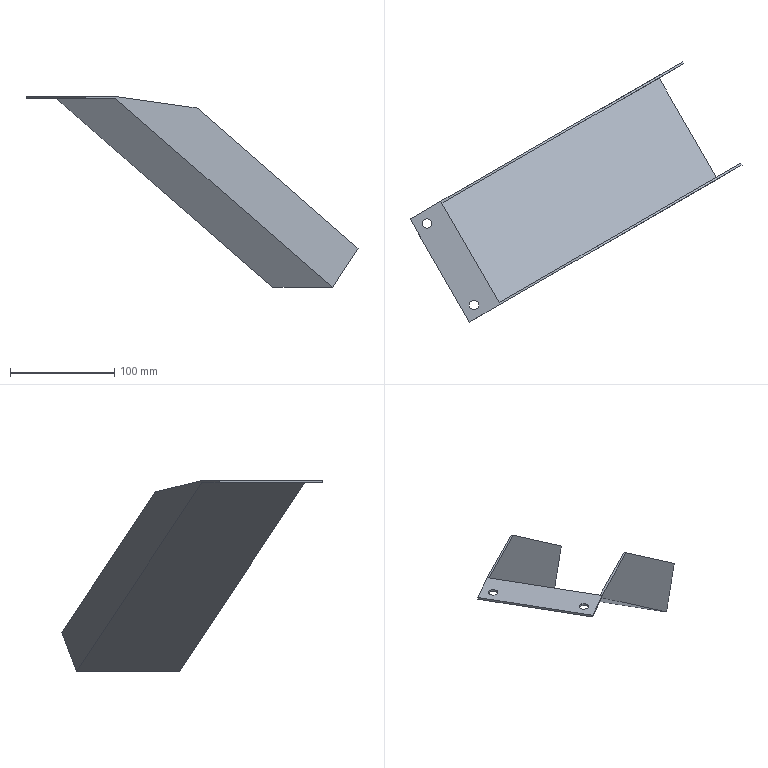Part | STEP file | lll_id4638_x_t | 1 solid | 16 faces | box 317.975 x 249.401 x 182.62 mm | volume 123072 mm3 | plane 14 | cylinder 2 | commonest cylinder face diameters 9 x2
STEP:
#1=CARTESIAN_POINT('',(342.336,-335.291,-180.));
#2=VERTEX_POINT('',#1);
#3=CARTESIAN_POINT('',(550.377,-215.179,-361.023));
#4=VERTEX_POINT('',#3);
#5=CARTESIAN_POINT('',(465.997,-263.896,-287.601));
#6=DIRECTION('',(0.6916,0.3993,-0.6018));
#7=VECTOR('',#6,1.);
#8=LINE('',#5,#7);
#9=EDGE_CURVE('',#2,#4,#8,.T.);
#10=ORIENTED_EDGE('',*,*,#9,.F.);
#11=CARTESIAN_POINT('',(397.336,-430.554,-180.));
#12=VERTEX_POINT('',#11);
#13=CARTESIAN_POINT('',(304.836,-270.34,-180.));
#14=DIRECTION('',(0.5,-0.866,0.));
#15=VECTOR('',#14,1.);
#16=LINE('',#13,#15);
#17=EDGE_CURVE('',#2,#12,#16,.T.);
#18=ORIENTED_EDGE('',*,*,#17,.T.);
#19=CARTESIAN_POINT('',(605.377,-310.442,-361.023));
#20=VERTEX_POINT('',#19);
#21=CARTESIAN_POINT('',(520.997,-359.159,-287.601));
#22=DIRECTION('',(0.6916,0.3993,-0.6018));
#23=VECTOR('',#22,1.);
#24=LINE('',#21,#23);
#25=EDGE_CURVE('',#12,#20,#24,.T.);
#26=ORIENTED_EDGE('',*,*,#25,.T.);
#27=CARTESIAN_POINT('',(512.877,-150.227,-361.023));
#28=DIRECTION('',(0.5,-0.866,0.));
#29=VECTOR('',#28,1.);
#30=LINE('',#27,#29);
#31=EDGE_CURVE('',#4,#20,#30,.T.);
#32=ORIENTED_EDGE('',*,*,#31,.F.);
#33=EDGE_LOOP('',(#10,#18,#26,#32));
#34=FACE_OUTER_BOUND('',#33,.T.);
#35=CARTESIAN_POINT('',(428.497,-198.944,-287.601));
#36=DIRECTION('',(-0.5212,-0.3009,-0.7986));
#37=DIRECTION('',(-0.6916,-0.3993,0.6018));
#38=AXIS2_PLACEMENT_3D('',#35,#36,#37);
#39=PLANE('',#38);
#40=ADVANCED_FACE('',(#34),#39,.F.);
#41=CARTESIAN_POINT('',(475.666,-387.64,-190.94));
#42=VERTEX_POINT('',#41);
#43=CARTESIAN_POINT('',(398.5,-432.192,-180.));
#44=VERTEX_POINT('',#43);
#45=CARTESIAN_POINT('',(531.435,-355.442,-198.847));
#46=DIRECTION('',(-0.8596,-0.4963,0.1219));
#47=VECTOR('',#46,1.);
#48=LINE('',#45,#47);
#49=EDGE_CURVE('',#42,#44,#48,.T.);
#50=ORIENTED_EDGE('',*,*,#49,.T.);
#51=CARTESIAN_POINT('',(368.856,-449.307,-180.));
#52=VERTEX_POINT('',#51);
#53=CARTESIAN_POINT('',(521.997,-360.891,-180.));
#54=DIRECTION('',(-0.866,-0.5,0.));
#55=VECTOR('',#54,1.);
#56=LINE('',#53,#55);
#57=EDGE_CURVE('',#44,#52,#56,.T.);
#58=ORIENTED_EDGE('',*,*,#57,.T.);
#59=CARTESIAN_POINT('',(368.856,-449.307,-182.));
#60=VERTEX_POINT('',#59);
#61=CARTESIAN_POINT('',(368.856,-449.307,-180.));
#62=DIRECTION('',(0.,0.,-1.));
#63=VECTOR('',#62,1.);
#64=LINE('',#61,#63);
#65=EDGE_CURVE('',#52,#60,#64,.T.);
#66=ORIENTED_EDGE('',*,*,#65,.T.);
#67=CARTESIAN_POINT('',(397.757,-432.621,-182.));
#68=VERTEX_POINT('',#67);
#69=CARTESIAN_POINT('',(394.837,-434.307,-182.));
#70=DIRECTION('',(0.866,0.5,0.));
#71=VECTOR('',#70,1.);
#72=LINE('',#69,#71);
#73=EDGE_CURVE('',#60,#68,#72,.T.);
#74=ORIENTED_EDGE('',*,*,#73,.T.);
#75=CARTESIAN_POINT('',(605.335,-312.776,-362.62));
#76=VERTEX_POINT('',#75);
#77=CARTESIAN_POINT('',(520.955,-361.492,-289.198));
#78=DIRECTION('',(0.6916,0.3993,-0.6018));
#79=VECTOR('',#78,1.);
#80=LINE('',#77,#79);
#81=EDGE_CURVE('',#68,#76,#80,.T.);
#82=ORIENTED_EDGE('',*,*,#81,.T.);
#83=CARTESIAN_POINT('',(629.831,-298.633,-325.084));
#84=VERTEX_POINT('',#83);
#85=CARTESIAN_POINT('',(606.377,-312.174,-361.023));
#86=DIRECTION('',(-0.5212,-0.3009,-0.7986));
#87=VECTOR('',#86,1.);
#88=LINE('',#85,#87);
#89=EDGE_CURVE('',#84,#76,#88,.T.);
#90=ORIENTED_EDGE('',*,*,#89,.F.);
#91=CARTESIAN_POINT('',(545.451,-347.35,-251.662));
#92=DIRECTION('',(0.6916,0.3993,-0.6018));
#93=VECTOR('',#92,1.);
#94=LINE('',#91,#93);
#95=EDGE_CURVE('',#42,#84,#94,.T.);
#96=ORIENTED_EDGE('',*,*,#95,.F.);
#97=EDGE_LOOP('',(#50,#58,#66,#74,#82,#90,#96));
#98=FACE_OUTER_BOUND('',#97,.T.);
#99=CARTESIAN_POINT('',(521.997,-360.891,-287.601));
#100=DIRECTION('',(-0.5,0.866,0.));
#101=DIRECTION('',(-0.6916,-0.3993,0.6018));
#102=AXIS2_PLACEMENT_3D('',#99,#100,#101);
#103=PLANE('',#102);
#104=ADVANCED_FACE('',(#98),#103,.F.);
#105=CARTESIAN_POINT('',(397.5,-430.46,-180.));
#106=VERTEX_POINT('',#105);
#107=CARTESIAN_POINT('',(520.997,-359.159,-180.));
#108=DIRECTION('',(-0.866,-0.5,0.));
#109=VECTOR('',#108,1.);
#110=LINE('',#107,#109);
#111=EDGE_CURVE('',#106,#12,#110,.T.);
#112=ORIENTED_EDGE('',*,*,#111,.F.);
#113=CARTESIAN_POINT('',(474.666,-385.908,-190.94));
#114=VERTEX_POINT('',#113);
#115=CARTESIAN_POINT('',(530.435,-353.71,-198.847));
#116=DIRECTION('',(0.8596,0.4963,-0.1219));
#117=VECTOR('',#116,1.);
#118=LINE('',#115,#117);
#119=EDGE_CURVE('',#106,#114,#118,.T.);
#120=ORIENTED_EDGE('',*,*,#119,.T.);
#121=CARTESIAN_POINT('',(628.831,-296.901,-325.084));
#122=VERTEX_POINT('',#121);
#123=CARTESIAN_POINT('',(544.451,-345.618,-251.662));
#124=DIRECTION('',(0.6916,0.3993,-0.6018));
#125=VECTOR('',#124,1.);
#126=LINE('',#123,#125);
#127=EDGE_CURVE('',#114,#122,#126,.T.);
#128=ORIENTED_EDGE('',*,*,#127,.T.);
#129=CARTESIAN_POINT('',(605.377,-310.442,-361.023));
#130=DIRECTION('',(-0.5212,-0.3009,-0.7986));
#131=VECTOR('',#130,1.);
#132=LINE('',#129,#131);
#133=EDGE_CURVE('',#122,#20,#132,.T.);
#134=ORIENTED_EDGE('',*,*,#133,.T.);
#135=ORIENTED_EDGE('',*,*,#25,.F.);
#136=EDGE_LOOP('',(#112,#120,#128,#134,#135));
#137=FACE_OUTER_BOUND('',#136,.T.);
#138=CARTESIAN_POINT('',(520.997,-359.159,-287.601));
#139=DIRECTION('',(-0.5,0.866,0.));
#140=DIRECTION('',(-0.6916,-0.3993,0.6018));
#141=AXIS2_PLACEMENT_3D('',#138,#139,#140);
#142=PLANE('',#141);
#143=ADVANCED_FACE('',(#137),#142,.T.);
#144=CARTESIAN_POINT('',(341.5,-333.465,-180.));
#145=VERTEX_POINT('',#144);
#146=CARTESIAN_POINT('',(311.856,-350.58,-180.));
#147=VERTEX_POINT('',#146);
#148=CARTESIAN_POINT('',(475.431,-256.14,-180.));
#149=DIRECTION('',(-0.866,-0.5,0.));
#150=VECTOR('',#149,1.);
#151=LINE('',#148,#150);
#152=EDGE_CURVE('',#145,#147,#151,.T.);
#153=ORIENTED_EDGE('',*,*,#152,.F.);
#154=CARTESIAN_POINT('',(418.666,-288.913,-190.94));
#155=VERTEX_POINT('',#154);
#156=CARTESIAN_POINT('',(474.435,-256.715,-198.847));
#157=DIRECTION('',(-0.8596,-0.4963,0.1219));
#158=VECTOR('',#157,1.);
#159=LINE('',#156,#158);
#160=EDGE_CURVE('',#155,#145,#159,.T.);
#161=ORIENTED_EDGE('',*,*,#160,.F.);
#162=CARTESIAN_POINT('',(572.831,-199.906,-325.084));
#163=VERTEX_POINT('',#162);
#164=CARTESIAN_POINT('',(488.451,-248.623,-251.662));
#165=DIRECTION('',(0.6916,0.3993,-0.6018));
#166=VECTOR('',#165,1.);
#167=LINE('',#164,#166);
#168=EDGE_CURVE('',#155,#163,#167,.T.);
#169=ORIENTED_EDGE('',*,*,#168,.T.);
#170=CARTESIAN_POINT('',(548.335,-214.049,-362.62));
#171=VERTEX_POINT('',#170);
#172=CARTESIAN_POINT('',(549.377,-213.447,-361.023));
#173=DIRECTION('',(-0.5212,-0.3009,-0.7986));
#174=VECTOR('',#173,1.);
#175=LINE('',#172,#174);
#176=EDGE_CURVE('',#163,#171,#175,.T.);
#177=ORIENTED_EDGE('',*,*,#176,.T.);
#178=CARTESIAN_POINT('',(340.757,-333.894,-182.));
#179=VERTEX_POINT('',#178);
#180=CARTESIAN_POINT('',(463.955,-262.766,-289.198));
#181=DIRECTION('',(0.6916,0.3993,-0.6018));
#182=VECTOR('',#181,1.);
#183=LINE('',#180,#182);
#184=EDGE_CURVE('',#179,#171,#183,.T.);
#185=ORIENTED_EDGE('',*,*,#184,.F.);
#186=CARTESIAN_POINT('',(311.856,-350.58,-182.));
#187=VERTEX_POINT('',#186);
#188=CARTESIAN_POINT('',(337.837,-335.58,-182.));
#189=DIRECTION('',(-0.866,-0.5,0.));
#190=VECTOR('',#189,1.);
#191=LINE('',#188,#190);
#192=EDGE_CURVE('',#179,#187,#191,.T.);
#193=ORIENTED_EDGE('',*,*,#192,.T.);
#194=CARTESIAN_POINT('',(311.856,-350.58,-180.));
#195=DIRECTION('',(0.,0.,-1.));
#196=VECTOR('',#195,1.);
#197=LINE('',#194,#196);
#198=EDGE_CURVE('',#147,#187,#197,.T.);
#199=ORIENTED_EDGE('',*,*,#198,.F.);
#200=EDGE_LOOP('',(#153,#161,#169,#177,#185,#193,#199));
#201=FACE_OUTER_BOUND('',#200,.T.);
#202=CARTESIAN_POINT('',(464.997,-262.164,-287.601));
#203=DIRECTION('',(-0.5,0.866,0.));
#204=DIRECTION('',(-0.6916,-0.3993,0.6018));
#205=AXIS2_PLACEMENT_3D('',#202,#203,#204);
#206=PLANE('',#205);
#207=ADVANCED_FACE('',(#201),#206,.T.);
#208=CARTESIAN_POINT('',(419.666,-290.645,-190.94));
#209=VERTEX_POINT('',#208);
#210=CARTESIAN_POINT('',(342.5,-335.197,-180.));
#211=VERTEX_POINT('',#210);
#212=CARTESIAN_POINT('',(475.435,-258.447,-198.847));
#213=DIRECTION('',(-0.8596,-0.4963,0.1219));
#214=VECTOR('',#213,1.);
#215=LINE('',#212,#214);
#216=EDGE_CURVE('',#209,#211,#215,.T.);
#217=ORIENTED_EDGE('',*,*,#216,.T.);
#218=CARTESIAN_POINT('',(465.997,-263.896,-180.));
#219=DIRECTION('',(-0.866,-0.5,0.));
#220=VECTOR('',#219,1.);
#221=LINE('',#218,#220);
#222=EDGE_CURVE('',#211,#2,#221,.T.);
#223=ORIENTED_EDGE('',*,*,#222,.T.);
#224=ORIENTED_EDGE('',*,*,#9,.T.);
#225=CARTESIAN_POINT('',(573.831,-201.638,-325.084));
#226=VERTEX_POINT('',#225);
#227=CARTESIAN_POINT('',(550.377,-215.179,-361.023));
#228=DIRECTION('',(-0.5212,-0.3009,-0.7986));
#229=VECTOR('',#228,1.);
#230=LINE('',#227,#229);
#231=EDGE_CURVE('',#226,#4,#230,.T.);
#232=ORIENTED_EDGE('',*,*,#231,.F.);
#233=CARTESIAN_POINT('',(489.451,-250.355,-251.662));
#234=DIRECTION('',(0.6916,0.3993,-0.6018));
#235=VECTOR('',#234,1.);
#236=LINE('',#233,#235);
#237=EDGE_CURVE('',#209,#226,#236,.T.);
#238=ORIENTED_EDGE('',*,*,#237,.F.);
#239=EDGE_LOOP('',(#217,#223,#224,#232,#238));
#240=FACE_OUTER_BOUND('',#239,.T.);
#241=CARTESIAN_POINT('',(465.997,-263.896,-287.601));
#242=DIRECTION('',(-0.5,0.866,0.));
#243=DIRECTION('',(-0.6916,-0.3993,0.6018));
#244=AXIS2_PLACEMENT_3D('',#241,#242,#243);
#245=PLANE('',#244);
#246=ADVANCED_FACE('',(#240),#245,.F.);
#247=CARTESIAN_POINT('',(644.839,-858.864,-180.));
#248=DIRECTION('',(0.5,-0.866,0.));
#249=VECTOR('',#248,1.);
#250=LINE('',#247,#249);
#251=EDGE_CURVE('',#106,#44,#250,.T.);
#252=ORIENTED_EDGE('',*,*,#251,.T.);
#253=ORIENTED_EDGE('',*,*,#49,.F.);
#254=CARTESIAN_POINT('',(472.166,-381.578,-190.94));
#255=DIRECTION('',(-0.5,0.866,0.));
#256=VECTOR('',#255,1.);
#257=LINE('',#254,#256);
#258=EDGE_CURVE('',#42,#114,#257,.T.);
#259=ORIENTED_EDGE('',*,*,#258,.T.);
#260=ORIENTED_EDGE('',*,*,#119,.F.);
#261=EDGE_LOOP('',(#252,#253,#259,#260));
#262=FACE_OUTER_BOUND('',#261,.T.);
#263=CARTESIAN_POINT('',(2121.349,-6.401,-389.339));
#264=DIRECTION('',(-0.1055,-0.06093,-0.9925));
#265=DIRECTION('',(-0.9944,0.003228,0.1055));
#266=AXIS2_PLACEMENT_3D('',#263,#264,#265);
#267=PLANE('',#266);
#268=ADVANCED_FACE('',(#262),#267,.F.);
#269=CARTESIAN_POINT('',(644.839,-858.864,-180.));
#270=DIRECTION('',(0.5,-0.866,0.));
#271=VECTOR('',#270,1.);
#272=LINE('',#269,#271);
#273=EDGE_CURVE('',#145,#211,#272,.T.);
#274=ORIENTED_EDGE('',*,*,#273,.T.);
#275=ORIENTED_EDGE('',*,*,#216,.F.);
#276=CARTESIAN_POINT('',(722.005,-814.312,-190.94));
#277=DIRECTION('',(0.5,-0.866,0.));
#278=VECTOR('',#277,1.);
#279=LINE('',#276,#278);
#280=EDGE_CURVE('',#155,#209,#279,.T.);
#281=ORIENTED_EDGE('',*,*,#280,.F.);
#282=ORIENTED_EDGE('',*,*,#160,.T.);
#283=EDGE_LOOP('',(#274,#275,#281,#282));
#284=FACE_OUTER_BOUND('',#283,.T.);
#285=CARTESIAN_POINT('',(2121.349,-6.401,-389.339));
#286=DIRECTION('',(-0.1055,-0.06093,-0.9925));
#287=DIRECTION('',(-0.9944,0.003228,0.1055));
#288=AXIS2_PLACEMENT_3D('',#285,#286,#287);
#289=PLANE('',#288);
#290=ADVANCED_FACE('',(#284),#289,.F.);
#291=ORIENTED_EDGE('',*,*,#81,.F.);
#292=CARTESIAN_POINT('',(304.257,-270.674,-182.));
#293=DIRECTION('',(-0.5,0.866,0.));
#294=VECTOR('',#293,1.);
#295=LINE('',#292,#294);
#296=EDGE_CURVE('',#68,#179,#295,.T.);
#297=ORIENTED_EDGE('',*,*,#296,.T.);
#298=ORIENTED_EDGE('',*,*,#184,.T.);
#299=CARTESIAN_POINT('',(511.835,-150.829,-362.62));
#300=DIRECTION('',(0.5,-0.866,0.));
#301=VECTOR('',#300,1.);
#302=LINE('',#299,#301);
#303=EDGE_CURVE('',#171,#76,#302,.T.);
#304=ORIENTED_EDGE('',*,*,#303,.T.);
#305=EDGE_LOOP('',(#291,#297,#298,#304));
#306=FACE_OUTER_BOUND('',#305,.T.);
#307=CARTESIAN_POINT('',(427.455,-199.546,-289.198));
#308=DIRECTION('',(-0.5212,-0.3009,-0.7986));
#309=DIRECTION('',(-0.6916,-0.3993,0.6018));
#310=AXIS2_PLACEMENT_3D('',#307,#308,#309);
#311=PLANE('',#310);
#312=ADVANCED_FACE('',(#306),#311,.T.);
#313=ORIENTED_EDGE('',*,*,#303,.F.);
#314=ORIENTED_EDGE('',*,*,#176,.F.);
#315=CARTESIAN_POINT('',(573.831,-201.638,-325.084));
#316=DIRECTION('',(-0.5,0.866,0.));
#317=VECTOR('',#316,1.);
#318=LINE('',#315,#317);
#319=EDGE_CURVE('',#226,#163,#318,.T.);
#320=ORIENTED_EDGE('',*,*,#319,.F.);
#321=ORIENTED_EDGE('',*,*,#231,.T.);
#322=ORIENTED_EDGE('',*,*,#31,.T.);
#323=ORIENTED_EDGE('',*,*,#133,.F.);
#324=CARTESIAN_POINT('',(536.331,-136.686,-325.084));
#325=DIRECTION('',(0.5,-0.866,0.));
#326=VECTOR('',#325,1.);
#327=LINE('',#324,#326);
#328=EDGE_CURVE('',#122,#84,#327,.T.);
#329=ORIENTED_EDGE('',*,*,#328,.T.);
#330=ORIENTED_EDGE('',*,*,#89,.T.);
#331=EDGE_LOOP('',(#313,#314,#320,#321,#322,#323,#329,#330));
#332=FACE_OUTER_BOUND('',#331,.T.);
#333=CARTESIAN_POINT('',(512.877,-150.227,-361.023));
#334=DIRECTION('',(-0.6916,-0.3993,0.6018));
#335=DIRECTION('',(0.5212,0.3009,0.7986));
#336=AXIS2_PLACEMENT_3D('',#333,#334,#335);
#337=PLANE('',#336);
#338=ADVANCED_FACE('',(#332),#337,.F.);
#339=ORIENTED_EDGE('',*,*,#258,.F.);
#340=ORIENTED_EDGE('',*,*,#95,.T.);
#341=ORIENTED_EDGE('',*,*,#328,.F.);
#342=ORIENTED_EDGE('',*,*,#127,.F.);
#343=EDGE_LOOP('',(#339,#340,#341,#342));
#344=FACE_OUTER_BOUND('',#343,.T.);
#345=CARTESIAN_POINT('',(541.951,-341.288,-251.662));
#346=DIRECTION('',(-0.5212,-0.3009,-0.7986));
#347=DIRECTION('',(-0.6916,-0.3993,0.6018));
#348=AXIS2_PLACEMENT_3D('',#345,#346,#347);
#349=PLANE('',#348);
#350=ADVANCED_FACE('',(#344),#349,.F.);
#351=ORIENTED_EDGE('',*,*,#280,.T.);
#352=ORIENTED_EDGE('',*,*,#237,.T.);
#353=ORIENTED_EDGE('',*,*,#319,.T.);
#354=ORIENTED_EDGE('',*,*,#168,.F.);
#355=EDGE_LOOP('',(#351,#352,#353,#354));
#356=FACE_OUTER_BOUND('',#355,.T.);
#357=CARTESIAN_POINT('',(489.451,-250.355,-251.662));
#358=DIRECTION('',(0.5212,0.3009,0.7986));
#359=DIRECTION('',(0.6916,0.3993,-0.6018));
#360=AXIS2_PLACEMENT_3D('',#357,#358,#359);
#361=PLANE('',#360);
#362=ADVANCED_FACE('',(#356),#361,.T.);
#363=CARTESIAN_POINT('',(323.748,-354.972,-180.));
#364=VERTEX_POINT('',#363);
#365=CARTESIAN_POINT('',(328.248,-354.972,-180.));
#366=DIRECTION('',(0.,0.,-1.));
#367=DIRECTION('',(-1.,0.,0.));
#368=AXIS2_PLACEMENT_3D('',#365,#366,#367);
#369=CIRCLE('',#368,4.5);
#370=EDGE_CURVE('',#364,#364,#369,.T.);
#371=ORIENTED_EDGE('',*,*,#370,.T.);
#372=EDGE_LOOP('',(#371));
#373=FACE_BOUND('',#372,.T.);
#374=CARTESIAN_POINT('',(368.748,-432.915,-180.));
#375=VERTEX_POINT('',#374);
#376=CARTESIAN_POINT('',(373.248,-432.915,-180.));
#377=DIRECTION('',(0.,0.,-1.));
#378=DIRECTION('',(-1.,0.,0.));
#379=AXIS2_PLACEMENT_3D('',#376,#377,#378);
#380=CIRCLE('',#379,4.5);
#381=EDGE_CURVE('',#375,#375,#380,.T.);
#382=ORIENTED_EDGE('',*,*,#381,.T.);
#383=EDGE_LOOP('',(#382));
#384=FACE_BOUND('',#383,.T.);
#385=CARTESIAN_POINT('',(366.356,-444.977,-180.));
#386=DIRECTION('',(0.5,-0.866,0.));
#387=VECTOR('',#386,1.);
#388=LINE('',#385,#387);
#389=EDGE_CURVE('',#147,#52,#388,.T.);
#390=ORIENTED_EDGE('',*,*,#389,.T.);
#391=ORIENTED_EDGE('',*,*,#57,.F.);
#392=ORIENTED_EDGE('',*,*,#251,.F.);
#393=ORIENTED_EDGE('',*,*,#111,.T.);
#394=ORIENTED_EDGE('',*,*,#17,.F.);
#395=ORIENTED_EDGE('',*,*,#222,.F.);
#396=ORIENTED_EDGE('',*,*,#273,.F.);
#397=ORIENTED_EDGE('',*,*,#152,.T.);
#398=EDGE_LOOP('',(#390,#391,#392,#393,#394,#395,#396,#397));
#399=FACE_BOUND('',#398,.T.);
#400=CARTESIAN_POINT('',(2132.435,0.,-180.));
#401=DIRECTION('',(0.,0.,-1.));
#402=DIRECTION('',(-1.,0.,0.));
#403=AXIS2_PLACEMENT_3D('',#400,#401,#402);
#404=PLANE('',#403);
#405=ADVANCED_FACE('',(#373,#384,#399),#404,.F.);
#406=ORIENTED_EDGE('',*,*,#65,.F.);
#407=ORIENTED_EDGE('',*,*,#389,.F.);
#408=ORIENTED_EDGE('',*,*,#198,.T.);
#409=CARTESIAN_POINT('',(366.356,-444.977,-182.));
#410=DIRECTION('',(0.5,-0.866,0.));
#411=VECTOR('',#410,1.);
#412=LINE('',#409,#411);
#413=EDGE_CURVE('',#187,#60,#412,.T.);
#414=ORIENTED_EDGE('',*,*,#413,.T.);
#415=EDGE_LOOP('',(#406,#407,#408,#414));
#416=FACE_OUTER_BOUND('',#415,.T.);
#417=CARTESIAN_POINT('',(366.356,-444.977,-180.));
#418=DIRECTION('',(0.866,0.5,0.));
#419=DIRECTION('',(-0.5,0.866,0.));
#420=AXIS2_PLACEMENT_3D('',#417,#418,#419);
#421=PLANE('',#420);
#422=ADVANCED_FACE('',(#416),#421,.F.);
#423=CARTESIAN_POINT('',(377.748,-432.915,-182.));
#424=VERTEX_POINT('',#423);
#425=CARTESIAN_POINT('',(373.248,-432.915,-182.));
#426=DIRECTION('',(0.,0.,1.));
#427=DIRECTION('',(1.,0.,0.));
#428=AXIS2_PLACEMENT_3D('',#425,#426,#427);
#429=CIRCLE('',#428,4.5);
#430=EDGE_CURVE('',#424,#424,#429,.T.);
#431=ORIENTED_EDGE('',*,*,#430,.F.);
#432=EDGE_LOOP('',(#431));
#433=FACE_BOUND('',#432,.T.);
#434=ORIENTED_EDGE('',*,*,#381,.F.);
#435=EDGE_LOOP('',(#434));
#436=FACE_BOUND('',#435,.T.);
#437=CARTESIAN_POINT('',(373.248,-432.915,-182.));
#438=DIRECTION('',(0.,0.,1.));
#439=DIRECTION('',(1.,0.,0.));
#440=AXIS2_PLACEMENT_3D('',#437,#438,#439);
#441=CYLINDRICAL_SURFACE('',#440,4.5);
#442=ADVANCED_FACE('',(#433,#436),#441,.F.);
#443=CARTESIAN_POINT('',(332.748,-354.972,-182.));
#444=VERTEX_POINT('',#443);
#445=CARTESIAN_POINT('',(328.248,-354.972,-182.));
#446=DIRECTION('',(0.,0.,1.));
#447=DIRECTION('',(1.,0.,0.));
#448=AXIS2_PLACEMENT_3D('',#445,#446,#447);
#449=CIRCLE('',#448,4.5);
#450=EDGE_CURVE('',#444,#444,#449,.T.);
#451=ORIENTED_EDGE('',*,*,#450,.F.);
#452=EDGE_LOOP('',(#451));
#453=FACE_BOUND('',#452,.T.);
#454=ORIENTED_EDGE('',*,*,#370,.F.);
#455=EDGE_LOOP('',(#454));
#456=FACE_BOUND('',#455,.T.);
#457=CARTESIAN_POINT('',(328.248,-354.972,-182.));
#458=DIRECTION('',(0.,0.,1.));
#459=DIRECTION('',(1.,0.,0.));
#460=AXIS2_PLACEMENT_3D('',#457,#458,#459);
#461=CYLINDRICAL_SURFACE('',#460,4.5);
#462=ADVANCED_FACE('',(#453,#456),#461,.F.);
#463=ORIENTED_EDGE('',*,*,#296,.F.);
#464=ORIENTED_EDGE('',*,*,#73,.F.);
#465=ORIENTED_EDGE('',*,*,#413,.F.);
#466=ORIENTED_EDGE('',*,*,#192,.F.);
#467=EDGE_LOOP('',(#463,#464,#465,#466));
#468=FACE_BOUND('',#467,.T.);
#469=ORIENTED_EDGE('',*,*,#450,.T.);
#470=EDGE_LOOP('',(#469));
#471=FACE_BOUND('',#470,.T.);
#472=ORIENTED_EDGE('',*,*,#430,.T.);
#473=EDGE_LOOP('',(#472));
#474=FACE_BOUND('',#473,.T.);
#475=CARTESIAN_POINT('',(392.337,-429.977,-182.));
#476=DIRECTION('',(0.,0.,1.));
#477=DIRECTION('',(1.,0.,0.));
#478=AXIS2_PLACEMENT_3D('',#475,#476,#477);
#479=PLANE('',#478);
#480=ADVANCED_FACE('',(#468,#471,#474),#479,.F.);
#481=CLOSED_SHELL('',(#40,#104,#143,#207,#246,#268,#290,#312,#338,#350,#362,#405,#422,#442,#462,#480));
#482=MANIFOLD_SOLID_BREP('',#481);
#483=(LENGTH_UNIT()NAMED_UNIT(*)SI_UNIT(.MILLI.,.METRE.));
#484=UNCERTAINTY_MEASURE_WITH_UNIT(LENGTH_MEASURE(0.00002),#483,'','');
#485=(NAMED_UNIT(*)PLANE_ANGLE_UNIT()SI_UNIT($,.RADIAN.));
#486=PLANE_ANGLE_MEASURE_WITH_UNIT(PLANE_ANGLE_MEASURE(0.01745),#485);
#487=DIMENSIONAL_EXPONENTS(0.,0.,0.,0.,0.,0.,0.);
#488=(CONVERSION_BASED_UNIT('DEGREE',#486)NAMED_UNIT(#487)PLANE_ANGLE_UNIT());
#489=(NAMED_UNIT(*)SI_UNIT($,.STERADIAN.)SOLID_ANGLE_UNIT());
#490=(GEOMETRIC_REPRESENTATION_CONTEXT(3)GLOBAL_UNCERTAINTY_ASSIGNED_CONTEXT((#484))GLOBAL_UNIT_ASSIGNED_CONTEXT((#483,#488,#489))REPRESENTATION_CONTEXT('',''));
#491=ADVANCED_BREP_SHAPE_REPRESENTATION('',(#482),#490);